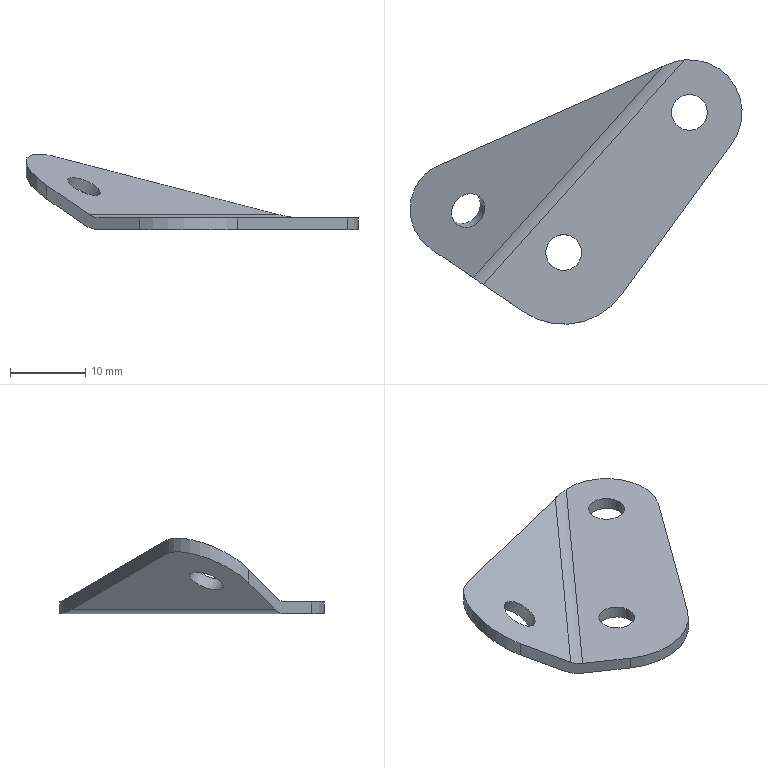Part | NX | features door hinge 2(left) 2 | 1 solid | 15 faces | box 44.096 x 35.138 x 10.064 mm | volume 1424 mm3 | cylinder 8 | plane 7 | commonest cylinder face diameters 4.763 x2 4.762 x1 6.35 x1 9.525 x1 12.7 x1 14 x1
STEP:
#1=CARTESIAN_POINT('',(-34.319,-18.136,7.273));
#2=VERTEX_POINT('',#1);
#3=CARTESIAN_POINT('',(-29.351,-21.517,3.834));
#4=VERTEX_POINT('',#3);
#5=CARTESIAN_POINT('',(-28.142,-22.341,2.997));
#6=DIRECTION('',(0.7175,-0.4884,-0.4967));
#7=VECTOR('',#6,1000.);
#8=LINE('',#5,#7);
#9=EDGE_CURVE('',#2,#4,#8,.T.);
#10=ORIENTED_EDGE('',*,*,#9,.F.);
#11=CARTESIAN_POINT('',(-33.314,-7.079,11.103));
#12=VERTEX_POINT('',#11);
#13=CARTESIAN_POINT('',(-30.746,-12.887,7.76));
#14=DIRECTION('',(-0.3723,0.3338,-0.866));
#15=DIRECTION('',(0.6448,-0.5782,-0.5));
#16=AXIS2_PLACEMENT_3D('',#13,#14,#15);
#17=ELLIPSE('',#16,7.332,6.35);
#18=EDGE_CURVE('',#12,#2,#17,.F.);
#19=ORIENTED_EDGE('',*,*,#18,.F.);
#20=CARTESIAN_POINT('',(-5.291,5.314,3.834));
#21=VERTEX_POINT('',#20);
#22=CARTESIAN_POINT('',(-5.435,5.25,3.871));
#23=DIRECTION('',(-0.8899,-0.3935,0.2308));
#24=VECTOR('',#23,1000.);
#25=LINE('',#22,#24);
#26=EDGE_CURVE('',#21,#12,#25,.T.);
#27=ORIENTED_EDGE('',*,*,#26,.F.);
#28=CARTESIAN_POINT('',(-137.75,-142.403,3.834));
#29=DIRECTION('',(0.6676,0.7445,0.));
#30=VECTOR('',#29,1000.);
#31=LINE('',#28,#30);
#32=EDGE_CURVE('',#4,#21,#31,.T.);
#33=ORIENTED_EDGE('',*,*,#32,.F.);
#34=EDGE_LOOP('',(#10,#19,#27,#33));
#35=FACE_BOUND('',#34,.T.);
#36=CARTESIAN_POINT('',(-32.148,-12.518,8.505));
#37=VERTEX_POINT('',#36);
#38=CARTESIAN_POINT('',(-29.961,-12.518,7.565));
#39=DIRECTION('',(-0.3723,0.3338,-0.866));
#40=DIRECTION('',(-0.9187,0.,0.3949));
#41=AXIS2_PLACEMENT_3D('',#38,#39,#40);
#42=CIRCLE('',#41,2.381);
#43=EDGE_CURVE('',#37,#37,#42,.T.);
#44=ORIENTED_EDGE('',*,*,#43,.F.);
#45=EDGE_LOOP('',(#44));
#46=FACE_BOUND('',#45,.T.);
#47=CARTESIAN_POINT('',(-136.927,-143.14,3.196));
#48=DIRECTION('',(0.3723,-0.3338,0.866));
#49=DIRECTION('',(-0.9187,0.,0.3949));
#50=AXIS2_PLACEMENT_3D('',#47,#48,#49);
#51=PLANE('',#50);
#52=ADVANCED_FACE('',(#35,#46),#51,.F.);
#53=CARTESIAN_POINT('',(-34.319,-18.136,9.106));
#54=VERTEX_POINT('',#53);
#55=CARTESIAN_POINT('',(-28.689,-21.968,5.209));
#56=VERTEX_POINT('',#55);
#57=CARTESIAN_POINT('',(-27.488,-22.785,4.378));
#58=DIRECTION('',(0.7175,-0.4884,-0.4967));
#59=VECTOR('',#58,1000.);
#60=LINE('',#57,#59);
#61=EDGE_CURVE('',#54,#56,#60,.T.);
#62=ORIENTED_EDGE('',*,*,#61,.T.);
#63=CARTESIAN_POINT('',(-3.524,6.095,5.209));
#64=VERTEX_POINT('',#63);
#65=CARTESIAN_POINT('',(-137.159,-142.932,5.209));
#66=DIRECTION('',(0.6676,0.7445,0.));
#67=VECTOR('',#66,1000.);
#68=LINE('',#65,#67);
#69=EDGE_CURVE('',#56,#64,#68,.T.);
#70=ORIENTED_EDGE('',*,*,#69,.T.);
#71=CARTESIAN_POINT('',(-33.314,-7.079,12.936));
#72=VERTEX_POINT('',#71);
#73=CARTESIAN_POINT('',(-5.059,5.417,5.607));
#74=DIRECTION('',(-0.8899,-0.3935,0.2308));
#75=VECTOR('',#74,1000.);
#76=LINE('',#73,#75);
#77=EDGE_CURVE('',#64,#72,#76,.T.);
#78=ORIENTED_EDGE('',*,*,#77,.T.);
#79=CARTESIAN_POINT('',(-30.746,-12.887,9.593));
#80=DIRECTION('',(-0.3723,0.3338,-0.866));
#81=DIRECTION('',(0.6448,-0.5782,-0.5));
#82=AXIS2_PLACEMENT_3D('',#79,#80,#81);
#83=ELLIPSE('',#82,7.332,6.35);
#84=EDGE_CURVE('',#72,#54,#83,.F.);
#85=ORIENTED_EDGE('',*,*,#84,.T.);
#86=EDGE_LOOP('',(#62,#70,#78,#85));
#87=FACE_BOUND('',#86,.T.);
#88=CARTESIAN_POINT('',(-31.557,-13.048,9.88));
#89=VERTEX_POINT('',#88);
#90=CARTESIAN_POINT('',(-29.37,-13.048,8.94));
#91=DIRECTION('',(-0.3723,0.3338,-0.866));
#92=DIRECTION('',(-0.9187,0.,0.3949));
#93=AXIS2_PLACEMENT_3D('',#90,#91,#92);
#94=CIRCLE('',#93,2.381);
#95=EDGE_CURVE('',#89,#89,#94,.F.);
#96=ORIENTED_EDGE('',*,*,#95,.F.);
#97=EDGE_LOOP('',(#96));
#98=FACE_BOUND('',#97,.T.);
#99=CARTESIAN_POINT('',(-136.336,-143.67,4.571));
#100=DIRECTION('',(0.3723,-0.3338,0.866));
#101=DIRECTION('',(-0.9187,0.,0.3949));
#102=AXIS2_PLACEMENT_3D('',#99,#100,#101);
#103=PLANE('',#102);
#104=ADVANCED_FACE('',(#87,#98),#103,.T.);
#105=CARTESIAN_POINT('',(-8.993,-24.223,4.783));
#106=VERTEX_POINT('',#105);
#107=CARTESIAN_POINT('',(-8.993,-24.223,3.196));
#108=VERTEX_POINT('',#107);
#109=CARTESIAN_POINT('',(-8.993,-24.223,15.875));
#110=DIRECTION('',(0.,0.,-1.));
#111=VECTOR('',#110,1000.);
#112=LINE('',#109,#111);
#113=EDGE_CURVE('',#106,#108,#112,.T.);
#114=ORIENTED_EDGE('',*,*,#113,.T.);
#115=CARTESIAN_POINT('',(5.657,-4.123,3.196));
#116=VERTEX_POINT('',#115);
#117=CARTESIAN_POINT('',(-8.993,-24.223,3.196));
#118=DIRECTION('',(0.589,0.8081,0.));
#119=VECTOR('',#118,1000.);
#120=LINE('',#117,#119);
#121=EDGE_CURVE('',#108,#116,#120,.T.);
#122=ORIENTED_EDGE('',*,*,#121,.T.);
#123=CARTESIAN_POINT('',(5.657,-4.123,4.783));
#124=VERTEX_POINT('',#123);
#125=CARTESIAN_POINT('',(5.657,-4.123,15.875));
#126=DIRECTION('',(0.,0.,-1.));
#127=VECTOR('',#126,1000.);
#128=LINE('',#125,#127);
#129=EDGE_CURVE('',#124,#116,#128,.T.);
#130=ORIENTED_EDGE('',*,*,#129,.F.);
#131=CARTESIAN_POINT('',(-8.993,-24.223,4.783));
#132=DIRECTION('',(0.589,0.8081,0.));
#133=VECTOR('',#132,1000.);
#134=LINE('',#131,#133);
#135=EDGE_CURVE('',#106,#124,#134,.T.);
#136=ORIENTED_EDGE('',*,*,#135,.F.);
#137=EDGE_LOOP('',(#114,#122,#130,#136));
#138=FACE_BOUND('',#137,.T.);
#139=CARTESIAN_POINT('',(-8.993,-24.223,15.875));
#140=DIRECTION('',(0.8081,-0.589,0.));
#141=DIRECTION('',(0.589,0.8081,0.));
#142=AXIS2_PLACEMENT_3D('',#139,#140,#141);
#143=PLANE('',#142);
#144=ADVANCED_FACE('',(#138),#143,.T.);
#145=CARTESIAN_POINT('',(-22.05,-26.487,4.783));
#146=VERTEX_POINT('',#145);
#147=CARTESIAN_POINT('',(-22.05,-26.487,3.196));
#148=VERTEX_POINT('',#147);
#149=CARTESIAN_POINT('',(-22.05,-26.487,15.875));
#150=DIRECTION('',(0.,0.,-1.));
#151=VECTOR('',#150,1000.);
#152=LINE('',#149,#151);
#153=EDGE_CURVE('',#146,#148,#152,.T.);
#154=ORIENTED_EDGE('',*,*,#153,.T.);
#155=CARTESIAN_POINT('',(-16.69,-18.613,3.196));
#156=DIRECTION('',(0.,0.,-1.));
#157=DIRECTION('',(-1.,0.,0.));
#158=AXIS2_PLACEMENT_3D('',#155,#156,#157);
#159=CIRCLE('',#158,9.525);
#160=EDGE_CURVE('',#148,#108,#159,.F.);
#161=ORIENTED_EDGE('',*,*,#160,.T.);
#162=ORIENTED_EDGE('',*,*,#113,.F.);
#163=CARTESIAN_POINT('',(-16.69,-18.613,4.783));
#164=DIRECTION('',(0.,0.,-1.));
#165=DIRECTION('',(-1.,0.,0.));
#166=AXIS2_PLACEMENT_3D('',#163,#164,#165);
#167=CIRCLE('',#166,9.525);
#168=EDGE_CURVE('',#146,#106,#167,.F.);
#169=ORIENTED_EDGE('',*,*,#168,.F.);
#170=EDGE_LOOP('',(#154,#161,#162,#169));
#171=FACE_BOUND('',#170,.T.);
#172=CARTESIAN_POINT('',(-16.69,-18.613,15.875));
#173=DIRECTION('',(0.,0.,-1.));
#174=DIRECTION('',(1.,0.,0.));
#175=AXIS2_PLACEMENT_3D('',#172,#173,#174);
#176=CYLINDRICAL_SURFACE('',#175,9.525);
#177=ADVANCED_FACE('',(#171),#176,.T.);
#178=CARTESIAN_POINT('',(-27.365,-22.869,4.783));
#179=VERTEX_POINT('',#178);
#180=CARTESIAN_POINT('',(-27.365,-22.869,7.958));
#181=DIRECTION('',(0.5627,0.8267,0.));
#182=DIRECTION('',(0.8267,-0.5627,0.));
#183=AXIS2_PLACEMENT_3D('',#180,#181,#182);
#184=ELLIPSE('',#183,3.203,3.175);
#185=EDGE_CURVE('',#179,#56,#184,.T.);
#186=ORIENTED_EDGE('',*,*,#185,.T.);
#187=ORIENTED_EDGE('',*,*,#61,.F.);
#188=CARTESIAN_POINT('',(-34.319,-18.136,15.875));
#189=DIRECTION('',(0.,0.,-1.));
#190=VECTOR('',#189,1000.);
#191=LINE('',#188,#190);
#192=EDGE_CURVE('',#54,#2,#191,.T.);
#193=ORIENTED_EDGE('',*,*,#192,.T.);
#194=ORIENTED_EDGE('',*,*,#9,.T.);
#195=CARTESIAN_POINT('',(-27.365,-22.869,3.196));
#196=VERTEX_POINT('',#195);
#197=CARTESIAN_POINT('',(-27.365,-22.869,7.958));
#198=DIRECTION('',(0.5627,0.8267,0.));
#199=DIRECTION('',(0.8267,-0.5627,0.));
#200=AXIS2_PLACEMENT_3D('',#197,#198,#199);
#201=ELLIPSE('',#200,4.805,4.763);
#202=EDGE_CURVE('',#196,#4,#201,.T.);
#203=ORIENTED_EDGE('',*,*,#202,.F.);
#204=CARTESIAN_POINT('',(-22.05,-26.487,3.196));
#205=DIRECTION('',(0.8267,-0.5627,0.));
#206=VECTOR('',#205,1000.);
#207=LINE('',#204,#206);
#208=EDGE_CURVE('',#196,#148,#207,.T.);
#209=ORIENTED_EDGE('',*,*,#208,.T.);
#210=ORIENTED_EDGE('',*,*,#153,.F.);
#211=CARTESIAN_POINT('',(-22.05,-26.487,4.783));
#212=DIRECTION('',(0.8267,-0.5627,0.));
#213=VECTOR('',#212,1000.);
#214=LINE('',#211,#213);
#215=EDGE_CURVE('',#179,#146,#214,.T.);
#216=ORIENTED_EDGE('',*,*,#215,.F.);
#217=EDGE_LOOP('',(#186,#187,#193,#194,#203,#209,#210,#216));
#218=FACE_BOUND('',#217,.T.);
#219=CARTESIAN_POINT('',(-22.05,-26.487,15.875));
#220=DIRECTION('',(-0.5627,-0.8267,0.));
#221=DIRECTION('',(0.8267,-0.5627,0.));
#222=AXIS2_PLACEMENT_3D('',#219,#220,#221);
#223=PLANE('',#222);
#224=ADVANCED_FACE('',(#218),#223,.T.);
#225=CARTESIAN_POINT('',(-33.314,-7.079,15.875));
#226=DIRECTION('',(0.,0.,-1.));
#227=VECTOR('',#226,1000.);
#228=LINE('',#225,#227);
#229=EDGE_CURVE('',#72,#12,#228,.T.);
#230=ORIENTED_EDGE('',*,*,#229,.T.);
#231=ORIENTED_EDGE('',*,*,#18,.T.);
#232=ORIENTED_EDGE('',*,*,#192,.F.);
#233=ORIENTED_EDGE('',*,*,#84,.F.);
#234=EDGE_LOOP('',(#230,#231,#232,#233));
#235=FACE_BOUND('',#234,.T.);
#236=CARTESIAN_POINT('',(-30.746,-12.887,15.875));
#237=DIRECTION('',(0.,0.,-1.));
#238=DIRECTION('',(1.,0.,0.));
#239=AXIS2_PLACEMENT_3D('',#236,#237,#238);
#240=CYLINDRICAL_SURFACE('',#239,6.35);
#241=ADVANCED_FACE('',(#235),#240,.T.);
#242=CARTESIAN_POINT('',(-2.831,6.402,5.051));
#243=VERTEX_POINT('',#242);
#244=CARTESIAN_POINT('',(0.009229,7.658,7.958));
#245=DIRECTION('',(0.4045,-0.9146,0.));
#246=DIRECTION('',(0.9146,0.4045,0.));
#247=AXIS2_PLACEMENT_3D('',#244,#245,#246);
#248=ELLIPSE('',#247,7.727,3.175);
#249=EDGE_CURVE('',#64,#243,#248,.T.);
#250=ORIENTED_EDGE('',*,*,#249,.T.);
#251=CARTESIAN_POINT('',(-2.831,6.402,3.37));
#252=VERTEX_POINT('',#251);
#253=CARTESIAN_POINT('',(-2.831,6.402,15.875));
#254=DIRECTION('',(0.,0.,-1.));
#255=VECTOR('',#254,1000.);
#256=LINE('',#253,#255);
#257=EDGE_CURVE('',#243,#252,#256,.T.);
#258=ORIENTED_EDGE('',*,*,#257,.T.);
#259=CARTESIAN_POINT('',(0.009229,7.658,7.958));
#260=DIRECTION('',(0.4045,-0.9146,0.));
#261=DIRECTION('',(0.9146,0.4045,0.));
#262=AXIS2_PLACEMENT_3D('',#259,#260,#261);
#263=ELLIPSE('',#262,11.591,4.763);
#264=EDGE_CURVE('',#21,#252,#263,.T.);
#265=ORIENTED_EDGE('',*,*,#264,.F.);
#266=ORIENTED_EDGE('',*,*,#26,.T.);
#267=ORIENTED_EDGE('',*,*,#229,.F.);
#268=ORIENTED_EDGE('',*,*,#77,.F.);
#269=EDGE_LOOP('',(#250,#258,#265,#266,#267,#268));
#270=FACE_BOUND('',#269,.T.);
#271=CARTESIAN_POINT('',(-2.831,6.402,15.875));
#272=DIRECTION('',(-0.4045,0.9146,0.));
#273=DIRECTION('',(-0.9146,-0.4045,0.));
#274=AXIS2_PLACEMENT_3D('',#271,#272,#273);
#275=PLANE('',#274);
#276=ADVANCED_FACE('',(#270),#275,.T.);
#277=CARTESIAN_POINT('',(-19.071,-18.613,3.196));
#278=VERTEX_POINT('',#277);
#279=CARTESIAN_POINT('',(-16.69,-18.613,3.196));
#280=DIRECTION('',(0.,0.,-1.));
#281=DIRECTION('',(-1.,0.,0.));
#282=AXIS2_PLACEMENT_3D('',#279,#280,#281);
#283=CIRCLE('',#282,2.381);
#284=EDGE_CURVE('',#278,#278,#283,.F.);
#285=ORIENTED_EDGE('',*,*,#284,.F.);
#286=EDGE_LOOP('',(#285));
#287=FACE_BOUND('',#286,.T.);
#288=CARTESIAN_POINT('',(-19.071,-18.613,4.783));
#289=VERTEX_POINT('',#288);
#290=CARTESIAN_POINT('',(-16.69,-18.613,4.783));
#291=DIRECTION('',(0.,0.,-1.));
#292=DIRECTION('',(-1.,0.,0.));
#293=AXIS2_PLACEMENT_3D('',#290,#291,#292);
#294=CIRCLE('',#293,2.381);
#295=EDGE_CURVE('',#289,#289,#294,.F.);
#296=ORIENTED_EDGE('',*,*,#295,.T.);
#297=EDGE_LOOP('',(#296));
#298=FACE_BOUND('',#297,.T.);
#299=CARTESIAN_POINT('',(-16.69,-18.613,15.875));
#300=DIRECTION('',(0.,0.,-1.));
#301=DIRECTION('',(1.,0.,0.));
#302=AXIS2_PLACEMENT_3D('',#299,#300,#301);
#303=CYLINDRICAL_SURFACE('',#302,2.381);
#304=ADVANCED_FACE('',(#287,#298),#303,.F.);
#305=CARTESIAN_POINT('',(-2.381,0.,3.196));
#306=VERTEX_POINT('',#305);
#307=CARTESIAN_POINT('',(0.,0.,3.196));
#308=DIRECTION('',(0.,0.,-1.));
#309=DIRECTION('',(-1.,0.,0.));
#310=AXIS2_PLACEMENT_3D('',#307,#308,#309);
#311=CIRCLE('',#310,2.381);
#312=EDGE_CURVE('',#306,#306,#311,.F.);
#313=ORIENTED_EDGE('',*,*,#312,.F.);
#314=EDGE_LOOP('',(#313));
#315=FACE_BOUND('',#314,.T.);
#316=CARTESIAN_POINT('',(-2.381,0.,4.783));
#317=VERTEX_POINT('',#316);
#318=CARTESIAN_POINT('',(0.,0.,4.783));
#319=DIRECTION('',(0.,0.,-1.));
#320=DIRECTION('',(-1.,0.,0.));
#321=AXIS2_PLACEMENT_3D('',#318,#319,#320);
#322=CIRCLE('',#321,2.381);
#323=EDGE_CURVE('',#317,#317,#322,.F.);
#324=ORIENTED_EDGE('',*,*,#323,.T.);
#325=EDGE_LOOP('',(#324));
#326=FACE_BOUND('',#325,.T.);
#327=CARTESIAN_POINT('',(0.,0.,15.875));
#328=DIRECTION('',(0.,0.,-1.));
#329=DIRECTION('',(1.,0.,0.));
#330=AXIS2_PLACEMENT_3D('',#327,#328,#329);
#331=CYLINDRICAL_SURFACE('',#330,2.381);
#332=ADVANCED_FACE('',(#315,#326),#331,.F.);
#333=CARTESIAN_POINT('',(-0.6043,6.974,4.783));
#334=VERTEX_POINT('',#333);
#335=CARTESIAN_POINT('',(-2.831,6.402,5.051));
#336=CARTESIAN_POINT('',(-2.126,6.714,4.912));
#337=CARTESIAN_POINT('',(-1.389,6.906,4.783));
#338=CARTESIAN_POINT('',(-0.6043,6.974,4.783));
#339=B_SPLINE_CURVE_WITH_KNOTS('',3,(#335,#336,#337,#338),.UNSPECIFIED.,.F.,.F.,(4,4),(0.,0.002315),.UNSPECIFIED.);
#340=EDGE_CURVE('',#243,#334,#339,.T.);
#341=ORIENTED_EDGE('',*,*,#340,.T.);
#342=CARTESIAN_POINT('',(0.,0.,4.783));
#343=DIRECTION('',(0.,0.,-1.));
#344=DIRECTION('',(-1.,0.,0.));
#345=AXIS2_PLACEMENT_3D('',#342,#343,#344);
#346=CIRCLE('',#345,7.);
#347=EDGE_CURVE('',#124,#334,#346,.F.);
#348=ORIENTED_EDGE('',*,*,#347,.F.);
#349=ORIENTED_EDGE('',*,*,#129,.T.);
#350=CARTESIAN_POINT('',(-0.6043,6.974,3.196));
#351=VERTEX_POINT('',#350);
#352=CARTESIAN_POINT('',(0.,0.,3.196));
#353=DIRECTION('',(0.,0.,-1.));
#354=DIRECTION('',(-1.,0.,0.));
#355=AXIS2_PLACEMENT_3D('',#352,#353,#354);
#356=CIRCLE('',#355,7.);
#357=EDGE_CURVE('',#116,#351,#356,.F.);
#358=ORIENTED_EDGE('',*,*,#357,.T.);
#359=CARTESIAN_POINT('',(-2.831,6.402,3.37));
#360=CARTESIAN_POINT('',(-2.123,6.715,3.282));
#361=CARTESIAN_POINT('',(-1.383,6.906,3.196));
#362=CARTESIAN_POINT('',(-0.6043,6.974,3.196));
#363=B_SPLINE_CURVE_WITH_KNOTS('',3,(#359,#360,#361,#362),.UNSPECIFIED.,.F.,.F.,(4,4),(0.,0.002306),.UNSPECIFIED.);
#364=EDGE_CURVE('',#252,#351,#363,.T.);
#365=ORIENTED_EDGE('',*,*,#364,.F.);
#366=ORIENTED_EDGE('',*,*,#257,.F.);
#367=EDGE_LOOP('',(#341,#348,#349,#358,#365,#366));
#368=FACE_BOUND('',#367,.T.);
#369=CARTESIAN_POINT('',(0.,0.,15.875));
#370=DIRECTION('',(0.,0.,-1.));
#371=DIRECTION('',(1.,0.,0.));
#372=AXIS2_PLACEMENT_3D('',#369,#370,#371);
#373=CYLINDRICAL_SURFACE('',#372,7.);
#374=ADVANCED_FACE('',(#368),#373,.T.);
#375=ORIENTED_EDGE('',*,*,#312,.T.);
#376=EDGE_LOOP('',(#375));
#377=FACE_BOUND('',#376,.T.);
#378=ORIENTED_EDGE('',*,*,#357,.F.);
#379=ORIENTED_EDGE('',*,*,#121,.F.);
#380=ORIENTED_EDGE('',*,*,#160,.F.);
#381=ORIENTED_EDGE('',*,*,#208,.F.);
#382=CARTESIAN_POINT('',(-135.977,-143.992,3.196));
#383=DIRECTION('',(0.6676,0.7445,0.));
#384=VECTOR('',#383,1000.);
#385=LINE('',#382,#384);
#386=EDGE_CURVE('',#351,#196,#385,.F.);
#387=ORIENTED_EDGE('',*,*,#386,.F.);
#388=EDGE_LOOP('',(#378,#379,#380,#381,#387));
#389=FACE_BOUND('',#388,.T.);
#390=ORIENTED_EDGE('',*,*,#284,.T.);
#391=EDGE_LOOP('',(#390));
#392=FACE_BOUND('',#391,.T.);
#393=CARTESIAN_POINT('',(-136.927,-143.14,3.196));
#394=DIRECTION('',(0.,0.,1.));
#395=DIRECTION('',(-1.,0.,0.));
#396=AXIS2_PLACEMENT_3D('',#393,#394,#395);
#397=PLANE('',#396);
#398=ADVANCED_FACE('',(#377,#389,#392),#397,.F.);
#399=ORIENTED_EDGE('',*,*,#202,.T.);
#400=ORIENTED_EDGE('',*,*,#32,.T.);
#401=ORIENTED_EDGE('',*,*,#264,.T.);
#402=ORIENTED_EDGE('',*,*,#364,.T.);
#403=ORIENTED_EDGE('',*,*,#386,.T.);
#404=EDGE_LOOP('',(#399,#400,#401,#402,#403));
#405=FACE_BOUND('',#404,.T.);
#406=CARTESIAN_POINT('',(-135.977,-143.992,7.958));
#407=DIRECTION('',(0.6676,0.7445,0.));
#408=DIRECTION('',(-0.7445,0.6676,0.));
#409=AXIS2_PLACEMENT_3D('',#406,#407,#408);
#410=CYLINDRICAL_SURFACE('',#409,4.763);
#411=ADVANCED_FACE('',(#405),#410,.T.);
#412=ORIENTED_EDGE('',*,*,#323,.F.);
#413=EDGE_LOOP('',(#412));
#414=FACE_BOUND('',#413,.T.);
#415=ORIENTED_EDGE('',*,*,#347,.T.);
#416=CARTESIAN_POINT('',(-135.977,-143.992,4.783));
#417=DIRECTION('',(0.6676,0.7445,0.));
#418=VECTOR('',#417,1000.);
#419=LINE('',#416,#418);
#420=EDGE_CURVE('',#334,#179,#419,.F.);
#421=ORIENTED_EDGE('',*,*,#420,.T.);
#422=ORIENTED_EDGE('',*,*,#215,.T.);
#423=ORIENTED_EDGE('',*,*,#168,.T.);
#424=ORIENTED_EDGE('',*,*,#135,.T.);
#425=EDGE_LOOP('',(#415,#421,#422,#423,#424));
#426=FACE_BOUND('',#425,.T.);
#427=ORIENTED_EDGE('',*,*,#295,.F.);
#428=EDGE_LOOP('',(#427));
#429=FACE_BOUND('',#428,.T.);
#430=CARTESIAN_POINT('',(-136.927,-143.14,4.783));
#431=DIRECTION('',(0.,0.,1.));
#432=DIRECTION('',(-1.,0.,0.));
#433=AXIS2_PLACEMENT_3D('',#430,#431,#432);
#434=PLANE('',#433);
#435=ADVANCED_FACE('',(#414,#426,#429),#434,.T.);
#436=ORIENTED_EDGE('',*,*,#185,.F.);
#437=ORIENTED_EDGE('',*,*,#420,.F.);
#438=ORIENTED_EDGE('',*,*,#340,.F.);
#439=ORIENTED_EDGE('',*,*,#249,.F.);
#440=ORIENTED_EDGE('',*,*,#69,.F.);
#441=EDGE_LOOP('',(#436,#437,#438,#439,#440));
#442=FACE_BOUND('',#441,.T.);
#443=CARTESIAN_POINT('',(-135.977,-143.992,7.958));
#444=DIRECTION('',(0.6676,0.7445,0.));
#445=DIRECTION('',(-0.7445,0.6676,0.));
#446=AXIS2_PLACEMENT_3D('',#443,#444,#445);
#447=CYLINDRICAL_SURFACE('',#446,3.175);
#448=ADVANCED_FACE('',(#442),#447,.F.);
#449=ORIENTED_EDGE('',*,*,#95,.T.);
#450=EDGE_LOOP('',(#449));
#451=FACE_BOUND('',#450,.T.);
#452=ORIENTED_EDGE('',*,*,#43,.T.);
#453=EDGE_LOOP('',(#452));
#454=FACE_BOUND('',#453,.T.);
#455=CARTESIAN_POINT('',(-25.233,-16.757,18.563));
#456=DIRECTION('',(-0.3723,0.3338,-0.866));
#457=DIRECTION('',(0.9187,0.,-0.3949));
#458=AXIS2_PLACEMENT_3D('',#455,#456,#457);
#459=CYLINDRICAL_SURFACE('',#458,2.381);
#460=ADVANCED_FACE('',(#451,#454),#459,.F.);
#461=CLOSED_SHELL('',(#52,#104,#144,#177,#224,#241,#276,#304,#332,#374,#398,#411,#435,#448,#460));
#462=MANIFOLD_SOLID_BREP('',#461);
#463=(LENGTH_UNIT()NAMED_UNIT(*)SI_UNIT(.MILLI.,.METRE.));
#464=UNCERTAINTY_MEASURE_WITH_UNIT(LENGTH_MEASURE(0.0508),#463,'','');
#465=(NAMED_UNIT(*)PLANE_ANGLE_UNIT()SI_UNIT($,.RADIAN.));
#466=(NAMED_UNIT(*)SI_UNIT($,.STERADIAN.)SOLID_ANGLE_UNIT());
#467=(GEOMETRIC_REPRESENTATION_CONTEXT(3)GLOBAL_UNCERTAINTY_ASSIGNED_CONTEXT((#464))GLOBAL_UNIT_ASSIGNED_CONTEXT((#463,#465,#466))REPRESENTATION_CONTEXT('',''));
#468=ADVANCED_BREP_SHAPE_REPRESENTATION('',(#462),#467);